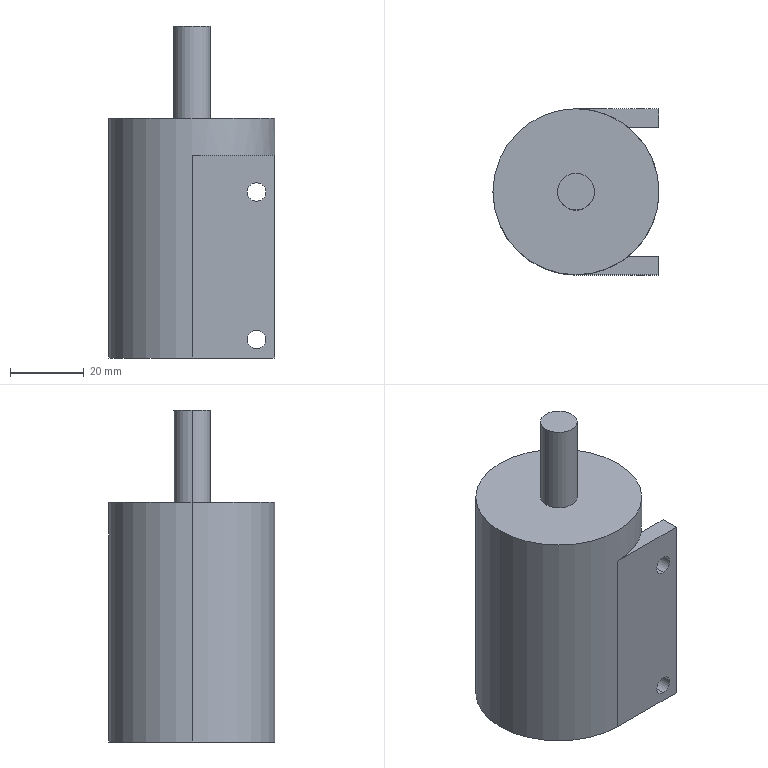Part | SolidWorks | features ICE 5, Extrusion 1 | 1 solid | 25 faces | box 45 x 45 x 90 mm | volume 73587 mm3 | plane 13 | cylinder 12 | commonest cylinder face diameters 5 x8 10 x2 45 x2
STEP:
#1=CARTESIAN_POINT('',(17.5,22.5,42.5));
#2=VERTEX_POINT('',#1);
#3=CARTESIAN_POINT('',(17.5,22.5,47.5));
#4=VERTEX_POINT('',#3);
#5=CARTESIAN_POINT('',(17.5,22.5,45.));
#6=DIRECTION('',(0.,1.,0.));
#7=DIRECTION('',(0.,0.,1.));
#8=AXIS2_PLACEMENT_3D('',#5,#6,#7);
#9=CIRCLE('',#8,2.5);
#10=EDGE_CURVE('',#2,#4,#9,.T.);
#11=ORIENTED_EDGE('',*,*,#10,.T.);
#12=CARTESIAN_POINT('',(17.5,17.5,47.5));
#13=VERTEX_POINT('',#12);
#14=CARTESIAN_POINT('',(17.5,37.5,47.5));
#15=DIRECTION('',(0.,-1.,0.));
#16=VECTOR('',#15,1000.);
#17=LINE('',#14,#16);
#18=EDGE_CURVE('',#4,#13,#17,.T.);
#19=ORIENTED_EDGE('',*,*,#18,.T.);
#20=CARTESIAN_POINT('',(17.5,17.5,42.5));
#21=VERTEX_POINT('',#20);
#22=CARTESIAN_POINT('',(17.5,17.5,45.));
#23=DIRECTION('',(0.,1.,0.));
#24=DIRECTION('',(0.,0.,1.));
#25=AXIS2_PLACEMENT_3D('',#22,#23,#24);
#26=CIRCLE('',#25,2.5);
#27=EDGE_CURVE('',#21,#13,#26,.T.);
#28=ORIENTED_EDGE('',*,*,#27,.F.);
#29=CARTESIAN_POINT('',(17.5,37.5,42.5));
#30=DIRECTION('',(0.,-1.,0.));
#31=VECTOR('',#30,1000.);
#32=LINE('',#29,#31);
#33=EDGE_CURVE('',#2,#21,#32,.T.);
#34=ORIENTED_EDGE('',*,*,#33,.F.);
#35=EDGE_LOOP('',(#11,#19,#28,#34));
#36=FACE_OUTER_BOUND('',#35,.T.);
#37=CARTESIAN_POINT('',(17.5,37.5,45.));
#38=DIRECTION('',(0.,-1.,0.));
#39=DIRECTION('',(0.,0.,-1.));
#40=AXIS2_PLACEMENT_3D('',#37,#38,#39);
#41=CYLINDRICAL_SURFACE('',#40,2.5);
#42=ADVANCED_FACE('',(#36),#41,.F.);
#43=CARTESIAN_POINT('',(17.5,-17.5,42.5));
#44=VERTEX_POINT('',#43);
#45=CARTESIAN_POINT('',(17.5,-17.5,47.5));
#46=VERTEX_POINT('',#45);
#47=CARTESIAN_POINT('',(17.5,-17.5,45.));
#48=DIRECTION('',(0.,1.,0.));
#49=DIRECTION('',(0.,0.,1.));
#50=AXIS2_PLACEMENT_3D('',#47,#48,#49);
#51=CIRCLE('',#50,2.5);
#52=EDGE_CURVE('',#44,#46,#51,.T.);
#53=ORIENTED_EDGE('',*,*,#52,.T.);
#54=CARTESIAN_POINT('',(17.5,-22.5,47.5));
#55=VERTEX_POINT('',#54);
#56=CARTESIAN_POINT('',(17.5,37.5,47.5));
#57=DIRECTION('',(0.,-1.,0.));
#58=VECTOR('',#57,1000.);
#59=LINE('',#56,#58);
#60=EDGE_CURVE('',#46,#55,#59,.T.);
#61=ORIENTED_EDGE('',*,*,#60,.T.);
#62=CARTESIAN_POINT('',(17.5,-22.5,42.5));
#63=VERTEX_POINT('',#62);
#64=CARTESIAN_POINT('',(17.5,-22.5,45.));
#65=DIRECTION('',(0.,-1.,0.));
#66=DIRECTION('',(0.,0.,-1.));
#67=AXIS2_PLACEMENT_3D('',#64,#65,#66);
#68=CIRCLE('',#67,2.5);
#69=EDGE_CURVE('',#55,#63,#68,.T.);
#70=ORIENTED_EDGE('',*,*,#69,.T.);
#71=CARTESIAN_POINT('',(17.5,37.5,42.5));
#72=DIRECTION('',(0.,-1.,0.));
#73=VECTOR('',#72,1000.);
#74=LINE('',#71,#73);
#75=EDGE_CURVE('',#44,#63,#74,.T.);
#76=ORIENTED_EDGE('',*,*,#75,.F.);
#77=EDGE_LOOP('',(#53,#61,#70,#76));
#78=FACE_OUTER_BOUND('',#77,.T.);
#79=CARTESIAN_POINT('',(17.5,37.5,45.));
#80=DIRECTION('',(0.,-1.,0.));
#81=DIRECTION('',(0.,0.,-1.));
#82=AXIS2_PLACEMENT_3D('',#79,#80,#81);
#83=CYLINDRICAL_SURFACE('',#82,2.5);
#84=ADVANCED_FACE('',(#78),#83,.F.);
#85=CARTESIAN_POINT('',(17.5,22.5,2.5));
#86=VERTEX_POINT('',#85);
#87=CARTESIAN_POINT('',(17.5,22.5,7.5));
#88=VERTEX_POINT('',#87);
#89=CARTESIAN_POINT('',(17.5,22.5,5.));
#90=DIRECTION('',(0.,1.,0.));
#91=DIRECTION('',(0.,0.,1.));
#92=AXIS2_PLACEMENT_3D('',#89,#90,#91);
#93=CIRCLE('',#92,2.5);
#94=EDGE_CURVE('',#86,#88,#93,.T.);
#95=ORIENTED_EDGE('',*,*,#94,.T.);
#96=CARTESIAN_POINT('',(17.5,17.5,7.5));
#97=VERTEX_POINT('',#96);
#98=CARTESIAN_POINT('',(17.5,37.5,7.5));
#99=DIRECTION('',(0.,-1.,0.));
#100=VECTOR('',#99,1000.);
#101=LINE('',#98,#100);
#102=EDGE_CURVE('',#88,#97,#101,.T.);
#103=ORIENTED_EDGE('',*,*,#102,.T.);
#104=CARTESIAN_POINT('',(17.5,17.5,2.5));
#105=VERTEX_POINT('',#104);
#106=CARTESIAN_POINT('',(17.5,17.5,5.));
#107=DIRECTION('',(0.,1.,0.));
#108=DIRECTION('',(0.,0.,1.));
#109=AXIS2_PLACEMENT_3D('',#106,#107,#108);
#110=CIRCLE('',#109,2.5);
#111=EDGE_CURVE('',#105,#97,#110,.T.);
#112=ORIENTED_EDGE('',*,*,#111,.F.);
#113=CARTESIAN_POINT('',(17.5,37.5,2.5));
#114=DIRECTION('',(0.,-1.,0.));
#115=VECTOR('',#114,1000.);
#116=LINE('',#113,#115);
#117=EDGE_CURVE('',#86,#105,#116,.T.);
#118=ORIENTED_EDGE('',*,*,#117,.F.);
#119=EDGE_LOOP('',(#95,#103,#112,#118));
#120=FACE_OUTER_BOUND('',#119,.T.);
#121=CARTESIAN_POINT('',(17.5,37.5,5.));
#122=DIRECTION('',(0.,-1.,0.));
#123=DIRECTION('',(0.,0.,-1.));
#124=AXIS2_PLACEMENT_3D('',#121,#122,#123);
#125=CYLINDRICAL_SURFACE('',#124,2.5);
#126=ADVANCED_FACE('',(#120),#125,.F.);
#127=CARTESIAN_POINT('',(17.5,-17.5,2.5));
#128=VERTEX_POINT('',#127);
#129=CARTESIAN_POINT('',(17.5,-17.5,7.5));
#130=VERTEX_POINT('',#129);
#131=CARTESIAN_POINT('',(17.5,-17.5,5.));
#132=DIRECTION('',(0.,1.,0.));
#133=DIRECTION('',(0.,0.,1.));
#134=AXIS2_PLACEMENT_3D('',#131,#132,#133);
#135=CIRCLE('',#134,2.5);
#136=EDGE_CURVE('',#128,#130,#135,.T.);
#137=ORIENTED_EDGE('',*,*,#136,.T.);
#138=CARTESIAN_POINT('',(17.5,-22.5,7.5));
#139=VERTEX_POINT('',#138);
#140=CARTESIAN_POINT('',(17.5,37.5,7.5));
#141=DIRECTION('',(0.,-1.,0.));
#142=VECTOR('',#141,1000.);
#143=LINE('',#140,#142);
#144=EDGE_CURVE('',#130,#139,#143,.T.);
#145=ORIENTED_EDGE('',*,*,#144,.T.);
#146=CARTESIAN_POINT('',(17.5,-22.5,2.5));
#147=VERTEX_POINT('',#146);
#148=CARTESIAN_POINT('',(17.5,-22.5,5.));
#149=DIRECTION('',(0.,-1.,0.));
#150=DIRECTION('',(0.,0.,-1.));
#151=AXIS2_PLACEMENT_3D('',#148,#149,#150);
#152=CIRCLE('',#151,2.5);
#153=EDGE_CURVE('',#139,#147,#152,.T.);
#154=ORIENTED_EDGE('',*,*,#153,.T.);
#155=CARTESIAN_POINT('',(17.5,37.5,2.5));
#156=DIRECTION('',(0.,-1.,0.));
#157=VECTOR('',#156,1000.);
#158=LINE('',#155,#157);
#159=EDGE_CURVE('',#128,#147,#158,.T.);
#160=ORIENTED_EDGE('',*,*,#159,.F.);
#161=EDGE_LOOP('',(#137,#145,#154,#160));
#162=FACE_OUTER_BOUND('',#161,.T.);
#163=CARTESIAN_POINT('',(17.5,37.5,5.));
#164=DIRECTION('',(0.,-1.,0.));
#165=DIRECTION('',(0.,0.,-1.));
#166=AXIS2_PLACEMENT_3D('',#163,#164,#165);
#167=CYLINDRICAL_SURFACE('',#166,2.5);
#168=ADVANCED_FACE('',(#162),#167,.F.);
#169=CARTESIAN_POINT('',(5.,0.,90.));
#170=VERTEX_POINT('',#169);
#171=CARTESIAN_POINT('',(-5.,0.,90.));
#172=VERTEX_POINT('',#171);
#173=CARTESIAN_POINT('',(0.,0.,90.));
#174=DIRECTION('',(0.,0.,1.));
#175=DIRECTION('',(1.,0.,0.));
#176=AXIS2_PLACEMENT_3D('',#173,#174,#175);
#177=CIRCLE('',#176,5.);
#178=EDGE_CURVE('',#170,#172,#177,.T.);
#179=ORIENTED_EDGE('',*,*,#178,.F.);
#180=CARTESIAN_POINT('',(5.,0.,65.));
#181=VERTEX_POINT('',#180);
#182=CARTESIAN_POINT('',(5.,0.,90.));
#183=DIRECTION('',(0.,0.,-1.));
#184=VECTOR('',#183,1000.);
#185=LINE('',#182,#184);
#186=EDGE_CURVE('',#170,#181,#185,.T.);
#187=ORIENTED_EDGE('',*,*,#186,.T.);
#188=CARTESIAN_POINT('',(-5.,0.,65.));
#189=VERTEX_POINT('',#188);
#190=CARTESIAN_POINT('',(0.,0.,65.));
#191=DIRECTION('',(0.,0.,1.));
#192=DIRECTION('',(1.,0.,0.));
#193=AXIS2_PLACEMENT_3D('',#190,#191,#192);
#194=CIRCLE('',#193,5.);
#195=EDGE_CURVE('',#181,#189,#194,.T.);
#196=ORIENTED_EDGE('',*,*,#195,.T.);
#197=CARTESIAN_POINT('',(-5.,0.,90.));
#198=DIRECTION('',(0.,0.,-1.));
#199=VECTOR('',#198,1000.);
#200=LINE('',#197,#199);
#201=EDGE_CURVE('',#172,#189,#200,.T.);
#202=ORIENTED_EDGE('',*,*,#201,.F.);
#203=EDGE_LOOP('',(#179,#187,#196,#202));
#204=FACE_OUTER_BOUND('',#203,.T.);
#205=CARTESIAN_POINT('',(0.,0.,90.));
#206=DIRECTION('',(0.,0.,-1.));
#207=DIRECTION('',(-1.,0.,0.));
#208=AXIS2_PLACEMENT_3D('',#205,#206,#207);
#209=CYLINDRICAL_SURFACE('',#208,5.);
#210=ADVANCED_FACE('',(#204),#209,.T.);
#211=CARTESIAN_POINT('',(22.5,0.,65.));
#212=VERTEX_POINT('',#211);
#213=CARTESIAN_POINT('',(-22.5,0.,65.));
#214=VERTEX_POINT('',#213);
#215=CARTESIAN_POINT('',(0.,0.,65.));
#216=DIRECTION('',(0.,0.,1.));
#217=DIRECTION('',(1.,0.,0.));
#218=AXIS2_PLACEMENT_3D('',#215,#216,#217);
#219=CIRCLE('',#218,22.5);
#220=EDGE_CURVE('',#212,#214,#219,.T.);
#221=ORIENTED_EDGE('',*,*,#220,.F.);
#222=CARTESIAN_POINT('',(22.5,0.,55.));
#223=VERTEX_POINT('',#222);
#224=CARTESIAN_POINT('',(22.5,0.,65.));
#225=DIRECTION('',(0.,0.,-1.));
#226=VECTOR('',#225,1000.);
#227=LINE('',#224,#226);
#228=EDGE_CURVE('',#212,#223,#227,.T.);
#229=ORIENTED_EDGE('',*,*,#228,.T.);
#230=CARTESIAN_POINT('',(14.142,17.5,55.));
#231=VERTEX_POINT('',#230);
#232=CARTESIAN_POINT('',(0.,0.,55.));
#233=DIRECTION('',(0.,0.,-1.));
#234=DIRECTION('',(-1.,0.,0.));
#235=AXIS2_PLACEMENT_3D('',#232,#233,#234);
#236=CIRCLE('',#235,22.5);
#237=EDGE_CURVE('',#231,#223,#236,.T.);
#238=ORIENTED_EDGE('',*,*,#237,.F.);
#239=CARTESIAN_POINT('',(0.,22.5,55.));
#240=VERTEX_POINT('',#239);
#241=CARTESIAN_POINT('',(0.,0.,55.));
#242=DIRECTION('',(0.,0.,1.));
#243=DIRECTION('',(1.,0.,0.));
#244=AXIS2_PLACEMENT_3D('',#241,#242,#243);
#245=CIRCLE('',#244,22.5);
#246=EDGE_CURVE('',#231,#240,#245,.T.);
#247=ORIENTED_EDGE('',*,*,#246,.T.);
#248=CARTESIAN_POINT('',(0.,22.5,0.));
#249=VERTEX_POINT('',#248);
#250=CARTESIAN_POINT('',(0.,22.5,0.));
#251=DIRECTION('',(0.,0.,1.));
#252=VECTOR('',#251,1000.);
#253=LINE('',#250,#252);
#254=EDGE_CURVE('',#249,#240,#253,.T.);
#255=ORIENTED_EDGE('',*,*,#254,.F.);
#256=CARTESIAN_POINT('',(-22.5,0.,0.));
#257=VERTEX_POINT('',#256);
#258=CARTESIAN_POINT('',(0.,0.,0.));
#259=DIRECTION('',(0.,0.,1.));
#260=DIRECTION('',(1.,0.,0.));
#261=AXIS2_PLACEMENT_3D('',#258,#259,#260);
#262=CIRCLE('',#261,22.5);
#263=EDGE_CURVE('',#249,#257,#262,.T.);
#264=ORIENTED_EDGE('',*,*,#263,.T.);
#265=CARTESIAN_POINT('',(-22.5,0.,65.));
#266=DIRECTION('',(0.,0.,-1.));
#267=VECTOR('',#266,1000.);
#268=LINE('',#265,#267);
#269=EDGE_CURVE('',#214,#257,#268,.T.);
#270=ORIENTED_EDGE('',*,*,#269,.F.);
#271=EDGE_LOOP('',(#221,#229,#238,#247,#255,#264,#270));
#272=FACE_OUTER_BOUND('',#271,.T.);
#273=CARTESIAN_POINT('',(0.,0.,65.));
#274=DIRECTION('',(0.,0.,-1.));
#275=DIRECTION('',(-1.,0.,0.));
#276=AXIS2_PLACEMENT_3D('',#273,#274,#275);
#277=CYLINDRICAL_SURFACE('',#276,22.5);
#278=ADVANCED_FACE('',(#272),#277,.T.);
#279=ORIENTED_EDGE('',*,*,#228,.F.);
#280=CARTESIAN_POINT('',(0.,0.,65.));
#281=DIRECTION('',(0.,0.,1.));
#282=DIRECTION('',(1.,0.,0.));
#283=AXIS2_PLACEMENT_3D('',#280,#281,#282);
#284=CIRCLE('',#283,22.5);
#285=EDGE_CURVE('',#214,#212,#284,.T.);
#286=ORIENTED_EDGE('',*,*,#285,.F.);
#287=ORIENTED_EDGE('',*,*,#269,.T.);
#288=CARTESIAN_POINT('',(0.,-22.5,0.));
#289=VERTEX_POINT('',#288);
#290=CARTESIAN_POINT('',(0.,0.,0.));
#291=DIRECTION('',(0.,0.,1.));
#292=DIRECTION('',(1.,0.,0.));
#293=AXIS2_PLACEMENT_3D('',#290,#291,#292);
#294=CIRCLE('',#293,22.5);
#295=EDGE_CURVE('',#257,#289,#294,.T.);
#296=ORIENTED_EDGE('',*,*,#295,.T.);
#297=CARTESIAN_POINT('',(0.,-22.5,55.));
#298=VERTEX_POINT('',#297);
#299=CARTESIAN_POINT('',(0.,-22.5,0.));
#300=DIRECTION('',(0.,0.,1.));
#301=VECTOR('',#300,1000.);
#302=LINE('',#299,#301);
#303=EDGE_CURVE('',#289,#298,#302,.T.);
#304=ORIENTED_EDGE('',*,*,#303,.T.);
#305=CARTESIAN_POINT('',(14.142,-17.5,55.));
#306=VERTEX_POINT('',#305);
#307=CARTESIAN_POINT('',(0.,0.,55.));
#308=DIRECTION('',(0.,0.,-1.));
#309=DIRECTION('',(-1.,0.,0.));
#310=AXIS2_PLACEMENT_3D('',#307,#308,#309);
#311=CIRCLE('',#310,22.5);
#312=EDGE_CURVE('',#306,#298,#311,.T.);
#313=ORIENTED_EDGE('',*,*,#312,.F.);
#314=CARTESIAN_POINT('',(0.,0.,55.));
#315=DIRECTION('',(0.,0.,-1.));
#316=DIRECTION('',(-1.,0.,0.));
#317=AXIS2_PLACEMENT_3D('',#314,#315,#316);
#318=CIRCLE('',#317,22.5);
#319=EDGE_CURVE('',#223,#306,#318,.T.);
#320=ORIENTED_EDGE('',*,*,#319,.F.);
#321=EDGE_LOOP('',(#279,#286,#287,#296,#304,#313,#320));
#322=FACE_OUTER_BOUND('',#321,.T.);
#323=CARTESIAN_POINT('',(0.,0.,65.));
#324=DIRECTION('',(0.,0.,-1.));
#325=DIRECTION('',(-1.,0.,0.));
#326=AXIS2_PLACEMENT_3D('',#323,#324,#325);
#327=CYLINDRICAL_SURFACE('',#326,22.5);
#328=ADVANCED_FACE('',(#322),#327,.T.);
#329=ORIENTED_EDGE('',*,*,#285,.T.);
#330=ORIENTED_EDGE('',*,*,#220,.T.);
#331=EDGE_LOOP('',(#329,#330));
#332=FACE_OUTER_BOUND('',#331,.T.);
#333=CARTESIAN_POINT('',(0.,0.,65.));
#334=DIRECTION('',(0.,0.,1.));
#335=DIRECTION('',(1.,0.,0.));
#336=AXIS2_PLACEMENT_3D('',#333,#334,#335);
#337=CIRCLE('',#336,5.);
#338=EDGE_CURVE('',#189,#181,#337,.T.);
#339=ORIENTED_EDGE('',*,*,#338,.F.);
#340=ORIENTED_EDGE('',*,*,#195,.F.);
#341=EDGE_LOOP('',(#339,#340));
#342=FACE_BOUND('',#341,.T.);
#343=CARTESIAN_POINT('',(0.,0.,65.));
#344=DIRECTION('',(0.,0.,1.));
#345=DIRECTION('',(1.,0.,0.));
#346=AXIS2_PLACEMENT_3D('',#343,#344,#345);
#347=PLANE('',#346);
#348=ADVANCED_FACE('',(#332,#342),#347,.T.);
#349=CARTESIAN_POINT('',(22.5,17.5,0.));
#350=VERTEX_POINT('',#349);
#351=CARTESIAN_POINT('',(0.,17.5,0.));
#352=VERTEX_POINT('',#351);
#353=CARTESIAN_POINT('',(0.,17.5,0.));
#354=DIRECTION('',(-1.,0.,0.));
#355=VECTOR('',#354,1000.);
#356=LINE('',#353,#355);
#357=EDGE_CURVE('',#350,#352,#356,.T.);
#358=ORIENTED_EDGE('',*,*,#357,.T.);
#359=CARTESIAN_POINT('',(0.,-17.5,0.));
#360=VERTEX_POINT('',#359);
#361=CARTESIAN_POINT('',(0.,-17.5,0.));
#362=DIRECTION('',(0.,1.,0.));
#363=VECTOR('',#362,1000.);
#364=LINE('',#361,#363);
#365=EDGE_CURVE('',#360,#352,#364,.T.);
#366=ORIENTED_EDGE('',*,*,#365,.F.);
#367=CARTESIAN_POINT('',(22.5,-17.5,0.));
#368=VERTEX_POINT('',#367);
#369=CARTESIAN_POINT('',(0.,-17.5,0.));
#370=DIRECTION('',(-1.,0.,0.));
#371=VECTOR('',#370,1000.);
#372=LINE('',#369,#371);
#373=EDGE_CURVE('',#368,#360,#372,.T.);
#374=ORIENTED_EDGE('',*,*,#373,.F.);
#375=CARTESIAN_POINT('',(22.5,-22.5,0.));
#376=VERTEX_POINT('',#375);
#377=CARTESIAN_POINT('',(22.5,-17.5,0.));
#378=DIRECTION('',(0.,-1.,0.));
#379=VECTOR('',#378,1000.);
#380=LINE('',#377,#379);
#381=EDGE_CURVE('',#368,#376,#380,.T.);
#382=ORIENTED_EDGE('',*,*,#381,.T.);
#383=CARTESIAN_POINT('',(0.,-22.5,0.));
#384=DIRECTION('',(-1.,0.,0.));
#385=VECTOR('',#384,1000.);
#386=LINE('',#383,#385);
#387=EDGE_CURVE('',#376,#289,#386,.T.);
#388=ORIENTED_EDGE('',*,*,#387,.T.);
#389=ORIENTED_EDGE('',*,*,#295,.F.);
#390=ORIENTED_EDGE('',*,*,#263,.F.);
#391=CARTESIAN_POINT('',(22.5,22.5,0.));
#392=VERTEX_POINT('',#391);
#393=CARTESIAN_POINT('',(0.,22.5,0.));
#394=DIRECTION('',(-1.,0.,0.));
#395=VECTOR('',#394,1000.);
#396=LINE('',#393,#395);
#397=EDGE_CURVE('',#392,#249,#396,.T.);
#398=ORIENTED_EDGE('',*,*,#397,.F.);
#399=CARTESIAN_POINT('',(22.5,17.5,0.));
#400=DIRECTION('',(0.,1.,0.));
#401=VECTOR('',#400,1000.);
#402=LINE('',#399,#401);
#403=EDGE_CURVE('',#350,#392,#402,.T.);
#404=ORIENTED_EDGE('',*,*,#403,.F.);
#405=EDGE_LOOP('',(#358,#366,#374,#382,#388,#389,#390,#398,#404));
#406=FACE_OUTER_BOUND('',#405,.T.);
#407=CARTESIAN_POINT('',(0.,0.,0.));
#408=DIRECTION('',(0.,0.,1.));
#409=DIRECTION('',(1.,0.,0.));
#410=AXIS2_PLACEMENT_3D('',#407,#408,#409);
#411=PLANE('',#410);
#412=ADVANCED_FACE('',(#406),#411,.F.);
#413=ORIENTED_EDGE('',*,*,#186,.F.);
#414=CARTESIAN_POINT('',(0.,0.,90.));
#415=DIRECTION('',(0.,0.,1.));
#416=DIRECTION('',(1.,0.,0.));
#417=AXIS2_PLACEMENT_3D('',#414,#415,#416);
#418=CIRCLE('',#417,5.);
#419=EDGE_CURVE('',#172,#170,#418,.T.);
#420=ORIENTED_EDGE('',*,*,#419,.F.);
#421=ORIENTED_EDGE('',*,*,#201,.T.);
#422=ORIENTED_EDGE('',*,*,#338,.T.);
#423=EDGE_LOOP('',(#413,#420,#421,#422));
#424=FACE_OUTER_BOUND('',#423,.T.);
#425=CARTESIAN_POINT('',(0.,0.,90.));
#426=DIRECTION('',(0.,0.,-1.));
#427=DIRECTION('',(-1.,0.,0.));
#428=AXIS2_PLACEMENT_3D('',#425,#426,#427);
#429=CYLINDRICAL_SURFACE('',#428,5.);
#430=ADVANCED_FACE('',(#424),#429,.T.);
#431=ORIENTED_EDGE('',*,*,#419,.T.);
#432=ORIENTED_EDGE('',*,*,#178,.T.);
#433=EDGE_LOOP('',(#431,#432));
#434=FACE_OUTER_BOUND('',#433,.T.);
#435=CARTESIAN_POINT('',(0.,0.,90.));
#436=DIRECTION('',(0.,0.,1.));
#437=DIRECTION('',(1.,0.,0.));
#438=AXIS2_PLACEMENT_3D('',#435,#436,#437);
#439=PLANE('',#438);
#440=ADVANCED_FACE('',(#434),#439,.T.);
#441=ORIENTED_EDGE('',*,*,#246,.F.);
#442=CARTESIAN_POINT('',(22.5,17.5,55.));
#443=VERTEX_POINT('',#442);
#444=CARTESIAN_POINT('',(0.,17.5,55.));
#445=DIRECTION('',(1.,0.,0.));
#446=VECTOR('',#445,1000.);
#447=LINE('',#444,#446);
#448=EDGE_CURVE('',#231,#443,#447,.T.);
#449=ORIENTED_EDGE('',*,*,#448,.T.);
#450=CARTESIAN_POINT('',(22.5,22.5,55.));
#451=VERTEX_POINT('',#450);
#452=CARTESIAN_POINT('',(22.5,17.5,55.));
#453=DIRECTION('',(0.,1.,0.));
#454=VECTOR('',#453,1000.);
#455=LINE('',#452,#454);
#456=EDGE_CURVE('',#443,#451,#455,.T.);
#457=ORIENTED_EDGE('',*,*,#456,.T.);
#458=CARTESIAN_POINT('',(0.,22.5,55.));
#459=DIRECTION('',(1.,0.,0.));
#460=VECTOR('',#459,1000.);
#461=LINE('',#458,#460);
#462=EDGE_CURVE('',#240,#451,#461,.T.);
#463=ORIENTED_EDGE('',*,*,#462,.F.);
#464=EDGE_LOOP('',(#441,#449,#457,#463));
#465=FACE_OUTER_BOUND('',#464,.T.);
#466=CARTESIAN_POINT('',(0.,17.5,55.));
#467=DIRECTION('',(0.,0.,1.));
#468=DIRECTION('',(1.,0.,0.));
#469=AXIS2_PLACEMENT_3D('',#466,#467,#468);
#470=PLANE('',#469);
#471=ADVANCED_FACE('',(#465),#470,.T.);
#472=ORIENTED_EDGE('',*,*,#27,.T.);
#473=CARTESIAN_POINT('',(17.5,17.5,45.));
#474=DIRECTION('',(0.,1.,0.));
#475=DIRECTION('',(0.,0.,1.));
#476=AXIS2_PLACEMENT_3D('',#473,#474,#475);
#477=CIRCLE('',#476,2.5);
#478=EDGE_CURVE('',#13,#21,#477,.T.);
#479=ORIENTED_EDGE('',*,*,#478,.T.);
#480=EDGE_LOOP('',(#472,#479));
#481=FACE_BOUND('',#480,.T.);
#482=ORIENTED_EDGE('',*,*,#111,.T.);
#483=CARTESIAN_POINT('',(17.5,17.5,5.));
#484=DIRECTION('',(0.,1.,0.));
#485=DIRECTION('',(0.,0.,1.));
#486=AXIS2_PLACEMENT_3D('',#483,#484,#485);
#487=CIRCLE('',#486,2.5);
#488=EDGE_CURVE('',#97,#105,#487,.T.);
#489=ORIENTED_EDGE('',*,*,#488,.T.);
#490=EDGE_LOOP('',(#482,#489));
#491=FACE_BOUND('',#490,.T.);
#492=ORIENTED_EDGE('',*,*,#448,.F.);
#493=CARTESIAN_POINT('',(0.,17.5,55.));
#494=VERTEX_POINT('',#493);
#495=CARTESIAN_POINT('',(0.,17.5,55.));
#496=DIRECTION('',(1.,0.,0.));
#497=VECTOR('',#496,1000.);
#498=LINE('',#495,#497);
#499=EDGE_CURVE('',#494,#231,#498,.T.);
#500=ORIENTED_EDGE('',*,*,#499,.F.);
#501=CARTESIAN_POINT('',(0.,17.5,55.));
#502=DIRECTION('',(0.,0.,-1.));
#503=VECTOR('',#502,1000.);
#504=LINE('',#501,#503);
#505=EDGE_CURVE('',#494,#352,#504,.T.);
#506=ORIENTED_EDGE('',*,*,#505,.T.);
#507=ORIENTED_EDGE('',*,*,#357,.F.);
#508=CARTESIAN_POINT('',(22.5,17.5,0.));
#509=DIRECTION('',(0.,0.,-1.));
#510=VECTOR('',#509,1000.);
#511=LINE('',#508,#510);
#512=EDGE_CURVE('',#443,#350,#511,.T.);
#513=ORIENTED_EDGE('',*,*,#512,.F.);
#514=EDGE_LOOP('',(#492,#500,#506,#507,#513));
#515=FACE_OUTER_BOUND('',#514,.T.);
#516=CARTESIAN_POINT('',(22.5,17.5,55.));
#517=DIRECTION('',(0.,1.,0.));
#518=DIRECTION('',(0.,0.,1.));
#519=AXIS2_PLACEMENT_3D('',#516,#517,#518);
#520=PLANE('',#519);
#521=ADVANCED_FACE('',(#481,#491,#515),#520,.F.);
#522=CARTESIAN_POINT('',(22.5,22.5,0.));
#523=DIRECTION('',(0.,0.,-1.));
#524=VECTOR('',#523,1000.);
#525=LINE('',#522,#524);
#526=EDGE_CURVE('',#451,#392,#525,.T.);
#527=ORIENTED_EDGE('',*,*,#526,.F.);
#528=ORIENTED_EDGE('',*,*,#456,.F.);
#529=ORIENTED_EDGE('',*,*,#512,.T.);
#530=ORIENTED_EDGE('',*,*,#403,.T.);
#531=EDGE_LOOP('',(#527,#528,#529,#530));
#532=FACE_OUTER_BOUND('',#531,.T.);
#533=CARTESIAN_POINT('',(22.5,17.5,0.));
#534=DIRECTION('',(1.,0.,0.));
#535=DIRECTION('',(0.,0.,-1.));
#536=AXIS2_PLACEMENT_3D('',#533,#534,#535);
#537=PLANE('',#536);
#538=ADVANCED_FACE('',(#532),#537,.T.);
#539=ORIENTED_EDGE('',*,*,#10,.F.);
#540=CARTESIAN_POINT('',(17.5,22.5,45.));
#541=DIRECTION('',(0.,1.,0.));
#542=DIRECTION('',(0.,0.,1.));
#543=AXIS2_PLACEMENT_3D('',#540,#541,#542);
#544=CIRCLE('',#543,2.5);
#545=EDGE_CURVE('',#4,#2,#544,.T.);
#546=ORIENTED_EDGE('',*,*,#545,.F.);
#547=EDGE_LOOP('',(#539,#546));
#548=FACE_BOUND('',#547,.T.);
#549=ORIENTED_EDGE('',*,*,#94,.F.);
#550=CARTESIAN_POINT('',(17.5,22.5,5.));
#551=DIRECTION('',(0.,1.,0.));
#552=DIRECTION('',(0.,0.,1.));
#553=AXIS2_PLACEMENT_3D('',#550,#551,#552);
#554=CIRCLE('',#553,2.5);
#555=EDGE_CURVE('',#88,#86,#554,.T.);
#556=ORIENTED_EDGE('',*,*,#555,.F.);
#557=EDGE_LOOP('',(#549,#556));
#558=FACE_BOUND('',#557,.T.);
#559=ORIENTED_EDGE('',*,*,#526,.T.);
#560=ORIENTED_EDGE('',*,*,#397,.T.);
#561=ORIENTED_EDGE('',*,*,#254,.T.);
#562=ORIENTED_EDGE('',*,*,#462,.T.);
#563=EDGE_LOOP('',(#559,#560,#561,#562));
#564=FACE_OUTER_BOUND('',#563,.T.);
#565=CARTESIAN_POINT('',(22.5,22.5,55.));
#566=DIRECTION('',(0.,1.,0.));
#567=DIRECTION('',(0.,0.,1.));
#568=AXIS2_PLACEMENT_3D('',#565,#566,#567);
#569=PLANE('',#568);
#570=ADVANCED_FACE('',(#548,#558,#564),#569,.T.);
#571=CARTESIAN_POINT('',(22.5,-17.5,55.));
#572=VERTEX_POINT('',#571);
#573=CARTESIAN_POINT('',(0.,-17.5,55.));
#574=DIRECTION('',(1.,0.,0.));
#575=VECTOR('',#574,1000.);
#576=LINE('',#573,#575);
#577=EDGE_CURVE('',#306,#572,#576,.T.);
#578=ORIENTED_EDGE('',*,*,#577,.F.);
#579=ORIENTED_EDGE('',*,*,#312,.T.);
#580=CARTESIAN_POINT('',(22.5,-22.5,55.));
#581=VERTEX_POINT('',#580);
#582=CARTESIAN_POINT('',(0.,-22.5,55.));
#583=DIRECTION('',(1.,0.,0.));
#584=VECTOR('',#583,1000.);
#585=LINE('',#582,#584);
#586=EDGE_CURVE('',#298,#581,#585,.T.);
#587=ORIENTED_EDGE('',*,*,#586,.T.);
#588=CARTESIAN_POINT('',(22.5,-17.5,55.));
#589=DIRECTION('',(0.,-1.,0.));
#590=VECTOR('',#589,1000.);
#591=LINE('',#588,#590);
#592=EDGE_CURVE('',#572,#581,#591,.T.);
#593=ORIENTED_EDGE('',*,*,#592,.F.);
#594=EDGE_LOOP('',(#578,#579,#587,#593));
#595=FACE_OUTER_BOUND('',#594,.T.);
#596=CARTESIAN_POINT('',(0.,-17.5,55.));
#597=DIRECTION('',(0.,0.,-1.));
#598=DIRECTION('',(-1.,0.,0.));
#599=AXIS2_PLACEMENT_3D('',#596,#597,#598);
#600=PLANE('',#599);
#601=ADVANCED_FACE('',(#595),#600,.F.);
#602=ORIENTED_EDGE('',*,*,#52,.F.);
#603=CARTESIAN_POINT('',(17.5,-17.5,45.));
#604=DIRECTION('',(0.,1.,0.));
#605=DIRECTION('',(0.,0.,1.));
#606=AXIS2_PLACEMENT_3D('',#603,#604,#605);
#607=CIRCLE('',#606,2.5);
#608=EDGE_CURVE('',#46,#44,#607,.T.);
#609=ORIENTED_EDGE('',*,*,#608,.F.);
#610=EDGE_LOOP('',(#602,#609));
#611=FACE_BOUND('',#610,.T.);
#612=ORIENTED_EDGE('',*,*,#136,.F.);
#613=CARTESIAN_POINT('',(17.5,-17.5,5.));
#614=DIRECTION('',(0.,1.,0.));
#615=DIRECTION('',(0.,0.,1.));
#616=AXIS2_PLACEMENT_3D('',#613,#614,#615);
#617=CIRCLE('',#616,2.5);
#618=EDGE_CURVE('',#130,#128,#617,.T.);
#619=ORIENTED_EDGE('',*,*,#618,.F.);
#620=EDGE_LOOP('',(#612,#619));
#621=FACE_BOUND('',#620,.T.);
#622=ORIENTED_EDGE('',*,*,#373,.T.);
#623=CARTESIAN_POINT('',(0.,-17.5,55.));
#624=VERTEX_POINT('',#623);
#625=CARTESIAN_POINT('',(0.,-17.5,55.));
#626=DIRECTION('',(0.,0.,-1.));
#627=VECTOR('',#626,1000.);
#628=LINE('',#625,#627);
#629=EDGE_CURVE('',#624,#360,#628,.T.);
#630=ORIENTED_EDGE('',*,*,#629,.F.);
#631=CARTESIAN_POINT('',(14.142,-17.5,55.));
#632=DIRECTION('',(-1.,0.,0.));
#633=VECTOR('',#632,1000.);
#634=LINE('',#631,#633);
#635=EDGE_CURVE('',#306,#624,#634,.T.);
#636=ORIENTED_EDGE('',*,*,#635,.F.);
#637=ORIENTED_EDGE('',*,*,#577,.T.);
#638=CARTESIAN_POINT('',(22.5,-17.5,0.));
#639=DIRECTION('',(0.,0.,-1.));
#640=VECTOR('',#639,1000.);
#641=LINE('',#638,#640);
#642=EDGE_CURVE('',#572,#368,#641,.T.);
#643=ORIENTED_EDGE('',*,*,#642,.T.);
#644=EDGE_LOOP('',(#622,#630,#636,#637,#643));
#645=FACE_OUTER_BOUND('',#644,.T.);
#646=CARTESIAN_POINT('',(0.,-17.5,55.));
#647=DIRECTION('',(0.,1.,0.));
#648=DIRECTION('',(0.,0.,1.));
#649=AXIS2_PLACEMENT_3D('',#646,#647,#648);
#650=PLANE('',#649);
#651=ADVANCED_FACE('',(#611,#621,#645),#650,.T.);
#652=CARTESIAN_POINT('',(22.5,-22.5,0.));
#653=DIRECTION('',(0.,0.,-1.));
#654=VECTOR('',#653,1000.);
#655=LINE('',#652,#654);
#656=EDGE_CURVE('',#581,#376,#655,.T.);
#657=ORIENTED_EDGE('',*,*,#656,.T.);
#658=ORIENTED_EDGE('',*,*,#381,.F.);
#659=ORIENTED_EDGE('',*,*,#642,.F.);
#660=ORIENTED_EDGE('',*,*,#592,.T.);
#661=EDGE_LOOP('',(#657,#658,#659,#660));
#662=FACE_OUTER_BOUND('',#661,.T.);
#663=CARTESIAN_POINT('',(22.5,-17.5,0.));
#664=DIRECTION('',(-1.,0.,0.));
#665=DIRECTION('',(0.,0.,1.));
#666=AXIS2_PLACEMENT_3D('',#663,#664,#665);
#667=PLANE('',#666);
#668=ADVANCED_FACE('',(#662),#667,.F.);
#669=CARTESIAN_POINT('',(17.5,-22.5,45.));
#670=DIRECTION('',(0.,-1.,0.));
#671=DIRECTION('',(0.,0.,-1.));
#672=AXIS2_PLACEMENT_3D('',#669,#670,#671);
#673=CIRCLE('',#672,2.5);
#674=EDGE_CURVE('',#63,#55,#673,.T.);
#675=ORIENTED_EDGE('',*,*,#674,.F.);
#676=ORIENTED_EDGE('',*,*,#69,.F.);
#677=EDGE_LOOP('',(#675,#676));
#678=FACE_BOUND('',#677,.T.);
#679=CARTESIAN_POINT('',(17.5,-22.5,5.));
#680=DIRECTION('',(0.,-1.,0.));
#681=DIRECTION('',(0.,0.,-1.));
#682=AXIS2_PLACEMENT_3D('',#679,#680,#681);
#683=CIRCLE('',#682,2.5);
#684=EDGE_CURVE('',#147,#139,#683,.T.);
#685=ORIENTED_EDGE('',*,*,#684,.F.);
#686=ORIENTED_EDGE('',*,*,#153,.F.);
#687=EDGE_LOOP('',(#685,#686));
#688=FACE_BOUND('',#687,.T.);
#689=ORIENTED_EDGE('',*,*,#303,.F.);
#690=ORIENTED_EDGE('',*,*,#387,.F.);
#691=ORIENTED_EDGE('',*,*,#656,.F.);
#692=ORIENTED_EDGE('',*,*,#586,.F.);
#693=EDGE_LOOP('',(#689,#690,#691,#692));
#694=FACE_OUTER_BOUND('',#693,.T.);
#695=CARTESIAN_POINT('',(0.,-22.5,55.));
#696=DIRECTION('',(0.,1.,0.));
#697=DIRECTION('',(0.,0.,1.));
#698=AXIS2_PLACEMENT_3D('',#695,#696,#697);
#699=PLANE('',#698);
#700=ADVANCED_FACE('',(#678,#688,#694),#699,.F.);
#701=ORIENTED_EDGE('',*,*,#365,.T.);
#702=ORIENTED_EDGE('',*,*,#505,.F.);
#703=CARTESIAN_POINT('',(0.,-17.5,55.));
#704=DIRECTION('',(0.,1.,0.));
#705=VECTOR('',#704,1000.);
#706=LINE('',#703,#705);
#707=EDGE_CURVE('',#624,#494,#706,.T.);
#708=ORIENTED_EDGE('',*,*,#707,.F.);
#709=ORIENTED_EDGE('',*,*,#629,.T.);
#710=EDGE_LOOP('',(#701,#702,#708,#709));
#711=FACE_OUTER_BOUND('',#710,.T.);
#712=CARTESIAN_POINT('',(0.,-17.5,55.));
#713=DIRECTION('',(-1.,0.,0.));
#714=DIRECTION('',(0.,-1.,0.));
#715=AXIS2_PLACEMENT_3D('',#712,#713,#714);
#716=PLANE('',#715);
#717=ADVANCED_FACE('',(#711),#716,.F.);
#718=ORIENTED_EDGE('',*,*,#237,.T.);
#719=ORIENTED_EDGE('',*,*,#319,.T.);
#720=ORIENTED_EDGE('',*,*,#635,.T.);
#721=ORIENTED_EDGE('',*,*,#707,.T.);
#722=ORIENTED_EDGE('',*,*,#499,.T.);
#723=EDGE_LOOP('',(#718,#719,#720,#721,#722));
#724=FACE_OUTER_BOUND('',#723,.T.);
#725=CARTESIAN_POINT('',(0.,0.,55.));
#726=DIRECTION('',(0.,0.,-1.));
#727=DIRECTION('',(-1.,0.,0.));
#728=AXIS2_PLACEMENT_3D('',#725,#726,#727);
#729=PLANE('',#728);
#730=ADVANCED_FACE('',(#724),#729,.T.);
#731=ORIENTED_EDGE('',*,*,#144,.F.);
#732=ORIENTED_EDGE('',*,*,#618,.T.);
#733=ORIENTED_EDGE('',*,*,#159,.T.);
#734=ORIENTED_EDGE('',*,*,#684,.T.);
#735=EDGE_LOOP('',(#731,#732,#733,#734));
#736=FACE_OUTER_BOUND('',#735,.T.);
#737=CARTESIAN_POINT('',(17.5,37.5,5.));
#738=DIRECTION('',(0.,-1.,0.));
#739=DIRECTION('',(0.,0.,-1.));
#740=AXIS2_PLACEMENT_3D('',#737,#738,#739);
#741=CYLINDRICAL_SURFACE('',#740,2.5);
#742=ADVANCED_FACE('',(#736),#741,.F.);
#743=ORIENTED_EDGE('',*,*,#102,.F.);
#744=ORIENTED_EDGE('',*,*,#555,.T.);
#745=ORIENTED_EDGE('',*,*,#117,.T.);
#746=ORIENTED_EDGE('',*,*,#488,.F.);
#747=EDGE_LOOP('',(#743,#744,#745,#746));
#748=FACE_OUTER_BOUND('',#747,.T.);
#749=CARTESIAN_POINT('',(17.5,37.5,5.));
#750=DIRECTION('',(0.,-1.,0.));
#751=DIRECTION('',(0.,0.,-1.));
#752=AXIS2_PLACEMENT_3D('',#749,#750,#751);
#753=CYLINDRICAL_SURFACE('',#752,2.5);
#754=ADVANCED_FACE('',(#748),#753,.F.);
#755=ORIENTED_EDGE('',*,*,#60,.F.);
#756=ORIENTED_EDGE('',*,*,#608,.T.);
#757=ORIENTED_EDGE('',*,*,#75,.T.);
#758=ORIENTED_EDGE('',*,*,#674,.T.);
#759=EDGE_LOOP('',(#755,#756,#757,#758));
#760=FACE_OUTER_BOUND('',#759,.T.);
#761=CARTESIAN_POINT('',(17.5,37.5,45.));
#762=DIRECTION('',(0.,-1.,0.));
#763=DIRECTION('',(0.,0.,-1.));
#764=AXIS2_PLACEMENT_3D('',#761,#762,#763);
#765=CYLINDRICAL_SURFACE('',#764,2.5);
#766=ADVANCED_FACE('',(#760),#765,.F.);
#767=ORIENTED_EDGE('',*,*,#18,.F.);
#768=ORIENTED_EDGE('',*,*,#545,.T.);
#769=ORIENTED_EDGE('',*,*,#33,.T.);
#770=ORIENTED_EDGE('',*,*,#478,.F.);
#771=EDGE_LOOP('',(#767,#768,#769,#770));
#772=FACE_OUTER_BOUND('',#771,.T.);
#773=CARTESIAN_POINT('',(17.5,37.5,45.));
#774=DIRECTION('',(0.,-1.,0.));
#775=DIRECTION('',(0.,0.,-1.));
#776=AXIS2_PLACEMENT_3D('',#773,#774,#775);
#777=CYLINDRICAL_SURFACE('',#776,2.5);
#778=ADVANCED_FACE('',(#772),#777,.F.);
#779=CLOSED_SHELL('',(#42,#84,#126,#168,#210,#278,#328,#348,#412,#430,#440,#471,#521,#538,#570,#601,#651,#668,#700,#717,#730,#742,#754,#766,#778));
#780=MANIFOLD_SOLID_BREP('',#779);
#781=CARTESIAN_POINT('',(0.,0.,0.));
#782=DIRECTION('',(0.,0.,1.));
#783=DIRECTION('',(1.,0.,0.));
#784=AXIS2_PLACEMENT_3D('',#781,#782,#783);
#785=(LENGTH_UNIT()NAMED_UNIT(*)SI_UNIT(.MILLI.,.METRE.));
#786=UNCERTAINTY_MEASURE_WITH_UNIT(LENGTH_MEASURE(0.00001),#785,'','');
#787=(NAMED_UNIT(*)PLANE_ANGLE_UNIT()SI_UNIT($,.RADIAN.));
#788=(NAMED_UNIT(*)SI_UNIT($,.STERADIAN.)SOLID_ANGLE_UNIT());
#789=(GEOMETRIC_REPRESENTATION_CONTEXT(3)GLOBAL_UNCERTAINTY_ASSIGNED_CONTEXT((#786))GLOBAL_UNIT_ASSIGNED_CONTEXT((#785,#787,#788))REPRESENTATION_CONTEXT('',''));
#790=ADVANCED_BREP_SHAPE_REPRESENTATION('',(#780,#784),#789);